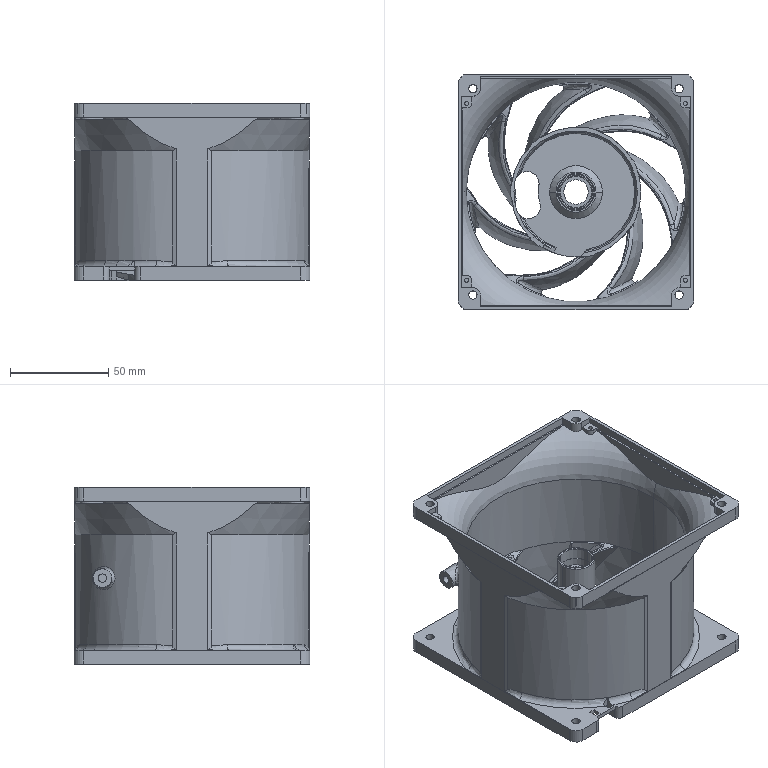NC program | NX | posted with a generic post | part box 120 x 120 x 90.2 mm
Lines 114333 to 115554 of 828686:
(等高精加工_COPY_COPY_COPY_COPY , TOOL : 2R0.2-柄4)
N228646 T09 M6
N228648 G54
N228650 G17 G0 G90 X-56.5 Y-45.575 S8000 M3
N228652 G43 Z140.7 H9
N228654 Z91.49
N228656 G94 G1 Z90.49 F1500.
N228658 X-56.759 Y-45.609
N228660 X-57. Y-45.709
N228662 X-57.207 Y-45.868
N228664 X-57.366 Y-46.075
N228666 X-57.466 Y-46.316
N228668 X-57.5 Y-46.575
N228670 Y-47.7
N228672 X-56.375
N228674 X-56.288 Z90.455
N228676 X-56.201 Z90.42
N228678 X-57.5
N228680 Y-46.401
N228682 Z90.35
N228684 Y-47.7
N228686 X-56.201
N228688 Z90.28
N228690 X-57.5
N228692 Y-46.401
N228694 Z90.21
N228696 Y-47.7
N228698 X-56.201
N228700 Z90.14
N228702 X-57.5
N228704 Y-46.401
N228706 Z90.07
N228708 Y-47.7
N228710 X-56.201
N228712 Z90.
N228714 X-57.5
N228716 Y-46.401
N228718 Z89.93
N228720 Y-47.7
N228722 X-56.201
N228724 Z89.86
N228726 X-57.5
N228728 Y-46.401
N228730 Z89.79
N228732 Y-47.7
N228734 X-56.201
N228736 Z89.72
N228738 X-57.5
N228740 Y-46.401
N228742 Z89.65
N228744 Y-47.7
N228746 X-56.201
N228748 Z89.58
N228750 X-57.5
N228752 Y-46.401
N228754 Z89.51
N228756 Y-47.7
N228758 X-56.201
N228760 Z89.44
N228762 X-57.5
N228764 Y-46.401
N228766 Z89.37
N228768 Y-47.7
N228770 X-56.201
N228772 Z89.3
N228774 X-57.5
N228776 Y-46.401
N228778 Z89.23
N228780 Y-47.7
N228782 X-56.201
N228784 Z89.16
N228786 X-57.5
N228788 Y-46.401
N228790 Z89.09
N228792 Y-47.7
N228794 X-56.201
N228796 Z89.02
N228798 X-57.5
N228800 Y-46.401
N228802 Z88.95
N228804 Y-47.7
N228806 X-56.201
N228808 Z88.88
N228810 X-57.5
N228812 Y-46.401
N228814 Z88.81
N228816 Y-47.7
N228818 X-56.201
N228820 Z88.74
N228822 X-57.5
N228824 Y-46.401
N228826 Z88.67
N228828 Y-47.7
N228830 X-56.201
N228832 Z88.6
N228834 X-57.5
N228836 Y-46.401
N228838 Z88.53
N228840 Y-47.7
N228842 X-56.201
N228844 Z88.46
N228846 X-57.5
N228848 Y-46.401
N228850 Z88.39
N228852 Y-47.7
N228854 X-56.201
N228856 Z88.32
N228858 X-57.5
N228860 Y-46.401
N228862 Z88.25
N228864 Y-47.7
N228866 X-56.201
N228868 Z88.18
N228870 X-57.5
N228872 Y-46.401
N228874 Z88.11
N228876 Y-47.7
N228878 X-56.201
N228880 Z88.04
N228882 X-57.5
N228884 Y-46.401
N228886 Z87.97
N228888 Y-47.7
N228890 X-56.201
N228892 Z87.9
N228894 X-57.5
N228896 Y-46.401
N228898 Z87.83
N228900 Y-47.7
N228902 X-56.201
N228904 Z87.76
N228906 X-57.5
N228908 Y-46.401
N228910 Z87.69
N228912 Y-47.7
N228914 X-56.201
N228916 Z87.62
N228918 X-57.5
N228920 Y-46.401
N228922 Z87.55
N228924 Y-47.7
N228926 X-56.201
N228928 Z87.48
N228930 X-57.5
N228932 Y-46.401
N228934 Z87.41
N228936 Y-47.7
N228938 X-56.201
N228940 Z87.34
N228942 X-57.5
N228944 Y-46.401
N228946 Z87.27
N228948 Y-47.7
N228950 X-56.201
N228952 Z87.2
N228954 X-57.5
N228956 Y-46.401
N228958 Z87.173
N228960 Y-47.7
N228962 X-56.201
N228964 Z87.125
N228966 X-57.5
N228968 Y-46.401
N228970 Z87.063
N228972 Y-47.7
N228974 X-56.201
N228976 Z86.994
N228978 X-57.5
N228980 Y-46.401
N228982 Z86.924
N228984 Y-47.7
N228986 X-56.201
N228988 Z86.854
N228990 X-57.5
N228992 Y-46.401
N228994 Z86.784
N228996 Y-47.7
N228998 X-56.201
N229000 Z86.714
N229002 X-57.5
N229004 Y-46.401
N229006 Z86.644
N229008 Y-47.7
N229010 X-56.201
N229012 X-55.942 Y-47.666
N229014 X-55.701 Y-47.566
N229016 X-55.494 Y-47.407
N229018 X-55.335 Y-47.2
N229020 X-55.235 Y-46.959
N229022 X-55.201 Y-46.7
N229024 Z87.644
N229026 G0 Z140.7
N229028 X-46.7 Y-55.375
N229030 Z91.49
N229032 G1 Z90.49
N229034 X-46.959 Y-55.409
N229036 X-47.2 Y-55.509
N229038 X-47.407 Y-55.668
N229040 X-47.566 Y-55.875
N229042 X-47.666 Y-56.116
N229044 X-47.7 Y-56.375
N229046 Y-57.5
N229048 X-46.575
N229050 X-46.488 Y-57.501 Z90.455
N229052 X-46.401 Y-57.5 Z90.42
N229054 X-47.7
N229056 Y-56.201
N229058 Z90.35
N229060 Y-57.5
N229062 X-46.401
N229064 Z90.28
N229066 X-47.7
N229068 Y-56.201
N229070 Z90.21
N229072 Y-57.5
N229074 X-46.401
N229076 Z90.14
N229078 X-47.7
N229080 Y-56.201
N229082 Z90.07
N229084 Y-57.5
N229086 X-46.401
N229088 Z90.
N229090 X-47.7
N229092 Y-56.201
N229094 Z89.93
N229096 Y-57.5
N229098 X-46.401
N229100 Z89.86
N229102 X-47.7
N229104 Y-56.201
N229106 Z89.79
N229108 Y-57.5
N229110 X-46.401
N229112 Z89.72
N229114 X-47.7
N229116 Y-56.201
N229118 Z89.65
N229120 Y-57.5
N229122 X-46.401
N229124 Z89.58
N229126 X-47.7
N229128 Y-56.201
N229130 Z89.51
N229132 Y-57.5
N229134 X-46.401
N229136 Z89.44
N229138 X-47.7
N229140 Y-56.201
N229142 Z89.37
N229144 Y-57.5
N229146 X-46.401
N229148 Z89.3
N229150 X-47.7
N229152 Y-56.201
N229154 Z89.23
N229156 Y-57.5
N229158 X-46.401
N229160 Z89.16
N229162 X-47.7
N229164 Y-56.201
N229166 Z89.09
N229168 Y-57.5
N229170 X-46.401
N229172 Z89.02
N229174 X-47.7
N229176 Y-56.201
N229178 Z88.95
N229180 Y-57.5
N229182 X-46.401
N229184 Z88.88
N229186 X-47.7
N229188 Y-56.201
N229190 Z88.81
N229192 Y-57.5
N229194 X-46.401
N229196 Z88.74
N229198 X-47.7
N229200 Y-56.201
N229202 Z88.67
N229204 Y-57.5
N229206 X-46.401
N229208 Z88.6
N229210 X-47.7
N229212 Y-56.201
N229214 Z88.53
N229216 Y-57.5
N229218 X-46.401
N229220 Z88.46
N229222 X-47.7
N229224 Y-56.201
N229226 Z88.39
N229228 Y-57.5
N229230 X-46.401
N229232 Z88.32
N229234 X-47.7
N229236 Y-56.201
N229238 Z88.25
N229240 Y-57.5
N229242 X-46.401
N229244 Z88.18
N229246 X-47.7
N229248 Y-56.201
N229250 Z88.11
N229252 Y-57.5
N229254 X-46.401
N229256 Z88.04
N229258 X-47.7
N229260 Y-56.201
N229262 Z87.97
N229264 Y-57.5
N229266 X-46.401
N229268 Z87.9
N229270 X-47.7
N229272 Y-56.201
N229274 Z87.83
N229276 Y-57.5
N229278 X-46.401
N229280 Z87.76
N229282 X-47.7
N229284 Y-56.201
N229286 Z87.69
N229288 Y-57.5
N229290 X-46.401
N229292 X-46.142 Y-57.466
N229294 X-45.901 Y-57.366
N229296 X-45.694 Y-57.207
N229298 X-45.535 Y-57.
N229300 X-45.435 Y-56.759
N229302 X-45.401 Y-56.5
N229304 Z88.69
N229306 G0 Z93.7
N229308 X-40.038
N229310 Z88.62
N229312 G1 Z87.62
N229314 X-40.072 Y-56.759
N229316 X-40.172 Y-57.
N229318 X-40.331 Y-57.207
N229320 X-40.538 Y-57.366
N229322 X-40.779 Y-57.466
N229324 X-41.038 Y-57.5
N229326 X-47.7
N229328 Y-52.7
N229330 X-47.734 Y-52.122
N229332 X-47.834 Y-51.552
N229334 X-47.851 Y-51.48 Z87.585
N229336 X-47.87 Y-51.409 Z87.55
N229338 X-47.776 Y-51.834
N229340 X-47.719 Y-52.265
N229342 X-47.7 Y-52.7
N229344 Y-57.5
N229346 X-40.865
N229348 X-40.78 Z87.48
N229350 X-47.7
N229352 Y-52.7
N229354 X-47.722 Y-52.232
N229356 X-47.788 Y-51.767
N229358 X-47.897 Y-51.311
N229360 X-47.918 Y-51.24 Z87.445
N229362 X-47.94 Y-51.17 Z87.41
N229364 X-47.807 Y-51.671
N229366 X-47.727 Y-52.183
N229368 X-47.7 Y-52.7
N229370 Y-57.5
N229372 X-40.63
N229374 X-40.544 Z87.34
N229376 X-47.7
N229378 Y-52.7
N229380 X-47.729 Y-52.158
N229382 X-47.817 Y-51.622
N229384 X-47.963 Y-51.1
N229386 X-47.979 Y-51.053 Z87.27
N229388 X-47.825 Y-51.59
N229390 X-47.731 Y-52.142
N229392 X-47.7 Y-52.7
N229394 Y-57.5
N229396 X-40.487
N229398 X-40.447 Z87.2
N229400 X-47.7
N229402 Y-52.7
N229404 X-47.733 Y-52.13
N229406 X-47.83 Y-51.568
N229408 X-47.991 Y-51.02
N229410 Z87.173
N229412 X-47.833 Y-51.553
N229414 X-47.736 Y-52.099
N229416 X-46.951
N229418 X-46.856 Y-52.067 Z87.149
N229420 X-46.761 Y-52.044 Z87.125
N229422 X-47.743
N229424 X-47.843 Y-51.515
N229426 X-47.998 Y-50.999
N229428 X-48.003 Y-50.987 Z87.063
N229430 X-47.848 Y-51.492
N229432 X-47.748 Y-52.01
N229434 X-46.814
N229436 X-46.823 Y-52. Z86.994
N229438 X-47.749
N229440 X-47.85 Y-51.485
N229442 X-48.004 Y-50.983
N229444 Z86.924
N229446 X-47.85 Y-51.485
N229448 X-47.749 Y-52.
N229450 X-46.647
N229452 Z86.854
N229454 X-47.749
N229456 X-47.85 Y-51.485
N229458 X-48.004 Y-50.983
N229460 Z86.784
N229462 X-47.85 Y-51.485
N229464 X-47.749 Y-52.
N229466 X-46.647
N229468 Z86.714
N229470 X-47.749
N229472 X-47.85 Y-51.485
N229474 X-48.004 Y-50.983
N229476 Z86.644
N229478 X-47.85 Y-51.485
N229480 X-47.749 Y-52.
N229482 X-46.647
N229484 Z86.574
N229486 X-47.749
N229488 X-47.85 Y-51.485
N229490 X-48.004 Y-50.983
N229492 Z86.504
N229494 X-47.85 Y-51.485
N229496 X-47.749 Y-52.
N229498 X-46.647
N229500 Z86.434
N229502 X-47.749
N229504 X-47.85 Y-51.485
N229506 X-48.004 Y-50.983
N229508 Z86.375
N229510 X-47.85 Y-51.485
N229512 X-47.749 Y-52.
N229514 X-46.647
N229516 Z86.317
N229518 X-47.749
N229520 X-47.85 Y-51.485
N229522 X-48.004 Y-50.983
N229524 Z86.258
N229526 X-47.85 Y-51.485
N229528 X-47.749 Y-52.
N229530 X-46.647
N229532 Z86.2
N229534 X-47.749
N229536 X-47.85 Y-51.485
N229538 X-48.004 Y-50.983
N229540 Z86.161
N229542 X-47.85 Y-51.485
N229544 X-47.749 Y-52.
N229546 X-46.647
N229548 Z86.108
N229550 X-47.749
N229552 X-47.85 Y-51.485
N229554 X-48.004 Y-50.983
N229556 Z86.043
N229558 X-47.85 Y-51.485
N229560 X-47.749 Y-52.
N229562 X-46.647
N229564 Z86.019
N229566 X-47.749
N229568 X-47.85 Y-51.485
N229570 X-48.004 Y-50.983
N229572 Z86.014
N229574 X-47.85 Y-51.485
N229576 X-47.749 Y-52.
N229578 X-46.647
N229580 Z86.01
N229582 X-47.749
N229584 X-47.85 Y-51.485
N229586 X-48.004 Y-50.983
N229588 Z86.005
N229590 X-47.85 Y-51.485
N229592 X-47.749 Y-52.
N229594 X-46.647
N229596 Z86.
N229598 X-47.749
N229600 X-47.85 Y-51.485
N229602 X-48.004 Y-50.983
N229604 Z85.995
N229606 X-47.85 Y-51.485
N229608 X-47.749 Y-52.
N229610 X-46.647
N229612 Z85.99
N229614 X-47.749
N229616 X-47.85 Y-51.485
N229618 X-48.004 Y-50.983
N229620 Z85.984
N229622 X-47.85 Y-51.485
N229624 X-47.749 Y-52.
N229626 X-46.647
N229628 Z85.978
N229630 X-47.749
N229632 X-47.85 Y-51.485
N229634 X-48.004 Y-50.983
N229636 Z85.972
N229638 X-47.85 Y-51.485
N229640 X-47.749 Y-52.
N229642 X-46.647
N229644 Z85.966
N229646 X-47.749
N229648 X-47.85 Y-51.485
N229650 X-48.004 Y-50.983
N229652 Z85.959
N229654 X-47.85 Y-51.485
N229656 X-47.749 Y-52.
N229658 X-46.647
N229660 Z85.952
N229662 X-47.749
N229664 X-47.85 Y-51.485
N229666 X-48.004 Y-50.983
N229668 Z85.945
N229670 X-47.85 Y-51.485
N229672 X-47.749 Y-52.
N229674 X-46.647
N229676 Z85.938
N229678 X-47.749
N229680 X-47.85 Y-51.485
N229682 X-48.004 Y-50.983
N229684 Z85.93
N229686 X-47.85 Y-51.485
N229688 X-47.749 Y-52.
N229690 X-46.647
N229692 Z85.922
N229694 X-47.749
N229696 X-47.85 Y-51.485
N229698 X-48.004 Y-50.983
N229700 Z85.914
N229702 X-47.85 Y-51.485
N229704 X-47.749 Y-52.
N229706 X-46.647
N229708 Z85.906
N229710 X-47.749
N229712 X-47.85 Y-51.485
N229714 X-48.004 Y-50.983
N229716 Z85.898
N229718 X-47.85 Y-51.485
N229720 X-47.749 Y-52.
N229722 X-46.647
N229724 Z85.889
N229726 X-47.749
N229728 X-47.85 Y-51.485
N229730 X-48.004 Y-50.983
N229732 Z85.88
N229734 X-47.85 Y-51.485
N229736 X-47.749 Y-52.
N229738 X-46.647
N229740 Z85.87
N229742 X-47.749
N229744 X-47.85 Y-51.485
N229746 X-48.004 Y-50.983
N229748 Z85.861
N229750 X-47.85 Y-51.485
N229752 X-47.749 Y-52.
N229754 X-46.647
N229756 Z85.851
N229758 X-47.749
N229760 X-47.85 Y-51.485
N229762 X-48.004 Y-50.983
N229764 Z85.841
N229766 X-47.85 Y-51.485
N229768 X-47.749 Y-52.
N229770 X-46.647
N229772 Z85.831
N229774 X-47.749
N229776 X-47.85 Y-51.485
N229778 X-48.004 Y-50.983
N229780 Z85.821
N229782 X-47.85 Y-51.485
N229784 X-47.749 Y-52.
N229786 X-46.647
N229788 Z85.81
N229790 X-47.749
N229792 X-47.85 Y-51.485
N229794 X-48.004 Y-50.983
N229796 Z85.799
N229798 X-47.85 Y-51.485
N229800 X-47.749 Y-52.
N229802 X-46.647
N229804 Z85.788
N229806 X-47.749
N229808 X-47.85 Y-51.485
N229810 X-48.004 Y-50.983
N229812 Z85.776
N229814 X-47.85 Y-51.485
N229816 X-47.749 Y-52.
N229818 X-46.647
N229820 Z85.765
N229822 X-47.749
N229824 X-47.85 Y-51.485
N229826 X-48.004 Y-50.983
N229828 Z85.753
N229830 X-47.85 Y-51.485
N229832 X-47.749 Y-52.
N229834 X-46.647
N229836 Z85.741
N229838 X-47.749
N229840 X-47.85 Y-51.485
N229842 X-48.004 Y-50.983
N229844 Z85.728
N229846 X-47.85 Y-51.485
N229848 X-47.749 Y-52.
N229850 X-46.647
N229852 Z85.716
N229854 X-47.749
N229856 X-47.85 Y-51.485
N229858 X-48.004 Y-50.983
N229860 X-48.008 Y-50.972 Z85.703
N229862 X-47.851 Y-51.479
N229864 X-47.749 Y-52.
N229866 X-46.636
N229868 X-46.587 Z85.69
N229870 X-47.749
N229872 X-47.858 Y-51.452
N229874 X-48.027 Y-50.92
N229876 X-48.048 Y-50.866 Z85.683
N229878 X-48.07 Y-50.812 Z85.676
N229880 X-47.873 Y-51.396
N229882 X-47.749 Y-52.
N229884 X-46.486
N229886 X-46.434 Z85.663
N229888 X-47.749
N229890 X-47.828 Y-51.576
N229892 X-47.943 Y-51.16
N229894 X-48.094 Y-50.755
N229896 X-48.12 Y-50.694 Z85.656
N229898 X-48.147 Y-50.633 Z85.649
N229900 X-47.971 Y-51.076
N229902 X-47.838 Y-51.533
N229904 X-47.749 Y-52.
N229906 X-46.326
N229908 X-46.271 Z85.635
N229910 X-47.749
N229912 X-47.844 Y-51.509
N229914 X-47.987 Y-51.031
N229916 X-48.177 Y-50.569
N229918 X-48.21 Y-50.5 Z85.628
N229920 X-48.245 Y-50.431 Z85.621
N229922 X-48.022 Y-50.935
N229924 X-47.856 Y-51.46
N229926 X-47.749 Y-52.
N229928 X-46.158
N229930 X-46.1 Z85.606
N229932 X-47.749
N229934 X-47.863 Y-51.433
N229936 X-48.042 Y-50.883
N229938 X-48.283 Y-50.357
N229940 X-48.325 Y-50.279 Z85.591
N229942 X-48.064 Y-50.828
N229944 X-47.871 Y-51.404
N229946 X-47.749 Y-52.
N229948 X-46.041
N229950 X-45.921 Z85.576
N229952 X-47.749
N229954 X-47.845 Y-51.504
N229956 X-47.99 Y-51.021
N229958 X-48.184 Y-50.555
N229960 X-48.423 Y-50.11
N229962 X-48.451 Y-50.064 Z85.569
N229964 X-48.481 Y-50.017 Z85.561
N229966 X-48.219 Y-50.481
N229968 X-48.009 Y-50.97
N229970 X-47.852 Y-51.478
N229972 X-47.749 Y-52.
N229974 X-45.86
N229976 X-45.798 Z85.546
N229978 X-47.749
N229980 X-47.859 Y-51.449
N229982 X-48.03 Y-50.914
N229984 X-48.26 Y-50.401
N229986 X-48.546 Y-49.917
N229988 X-48.584 Y-49.862 Z85.538
N229990 X-48.622 Y-49.807 Z85.53
N229992 X-48.315 Y-50.297
N229994 X-48.067 Y-50.82
N229996 X-47.881 Y-51.367
N229998 X-47.759 Y-51.932
N230000 X-47.722 Y-51.966
N230002 X-47.685 Y-52.
N230004 X-45.735
N230006 X-45.607 Z85.514
N230008 X-47.584
N230010 X-47.681 Y-51.911
N230012 X-47.778 Y-51.822
N230014 X-47.892 Y-51.328
N230016 X-48.056 Y-50.848
N230018 X-48.267 Y-50.387
N230020 X-48.524 Y-49.95
N230022 X-48.824 Y-49.541
N230024 X-48.873 Y-49.483 Z85.508
N230026 X-48.922 Y-49.424 Z85.503
N230028 X-48.973 Y-49.367 Z85.498
N230030 X-48.641 Y-49.78
N230032 X-48.355 Y-50.226
N230034 X-48.117 Y-50.7
N230036 X-47.932 Y-51.196
N230038 X-47.799 Y-51.709
N230040 X-47.641 Y-51.855
N230042 X-47.482 Y-52.
N230044 X-45.542
N230046 X-45.283 Y-51.966
N230048 X-45.042 Y-51.866
N230050 X-44.835 Y-51.707
N230052 X-44.676 Y-51.5
N230054 X-44.576 Y-51.259
N230056 X-44.542 Y-51.
N230058 Z86.498
N230060 G0 Z140.7
N230062 X-40.799 Y-55.529
N230064 Z88.173
N230066 G1 Z87.173
N230068 X-41.058 Y-55.564
N230070 X-41.299 Y-55.663
N230072 X-41.506 Y-55.822
N230074 X-41.665 Y-56.029
N230076 X-41.765 Y-56.271
N230078 X-41.799 Y-56.529
N230080 Y-57.5
N230082 X-40.447
N230084 X-40.421 Z87.125
N230086 X-41.744
N230088 Y-56.315
N230090 X-41.71 Y-56.368 Z87.063
N230092 Y-57.5
N230094 X-40.406
N230096 X-40.401 Z86.994
N230098 X-41.7
N230100 Y-56.377
N230102 Y-56.201 Z86.924
N230104 Y-57.5
N230106 X-40.401
N230108 Z86.854
N230110 X-41.7
N230112 Y-56.201
N230114 Z86.784
N230116 Y-57.5
N230118 X-40.401
N230120 Z86.714
N230122 X-41.7
N230124 Y-56.201
N230126 Z86.644
N230128 Y-57.5
N230130 X-40.401
N230132 X-40.142 Y-57.466
N230134 X-39.901 Y-57.366
N230136 X-39.694 Y-57.207
N230138 X-39.535 Y-57.
N230140 X-39.435 Y-56.759
N230142 X-39.401 Y-56.5
N230144 Z87.644
N230146 G0 Z140.7
N230148 X45.575
N230150 Z91.49
N230152 G1 Z90.49
N230154 X45.609 Y-56.759
N230156 X45.709 Y-57.
N230158 X45.868 Y-57.207
N230160 X46.075 Y-57.366
N230162 X46.316 Y-57.466
N230164 X46.575 Y-57.5
N230166 X47.7
N230168 Y-56.375
N230170 X47.701 Y-56.288 Z90.455
N230172 X47.7 Y-56.201 Z90.42
N230174 Y-57.5
N230176 X46.401
N230178 Z90.35
N230180 X47.7
N230182 Y-56.201
N230184 Z90.28
N230186 Y-57.5
N230188 X46.401
N230190 Z90.21
N230192 X47.7
N230194 Y-56.201
N230196 Z90.14
N230198 Y-57.5
N230200 X46.401
N230202 Z90.07
N230204 X47.7
N230206 Y-56.201
N230208 Z90.
N230210 Y-57.5
N230212 X46.401
N230214 Z89.93
N230216 X47.7
N230218 Y-56.201
N230220 Z89.86
N230222 Y-57.5
N230224 X46.401
N230226 Z89.79
N230228 X47.7
N230230 Y-56.201
N230232 Z89.72
N230234 Y-57.5
N230236 X46.401
N230238 Z89.65
N230240 X47.7
N230242 Y-56.201
N230244 Z89.58
N230246 Y-57.5
N230248 X46.401
N230250 Z89.51
N230252 X47.7
N230254 Y-56.201
N230256 Z89.44
N230258 Y-57.5
N230260 X46.401
N230262 Z89.37
N230264 X47.7
N230266 Y-56.201
N230268 Z89.3
N230270 Y-57.5
N230272 X46.401
N230274 Z89.23
N230276 X47.7
N230278 Y-56.201
N230280 Z89.16
N230282 Y-57.5
N230284 X46.401
N230286 Z89.09
N230288 X47.7
N230290 Y-56.201
N230292 Z89.02
N230294 Y-57.5
N230296 X46.401
N230298 Z88.95
N230300 X47.7
N230302 Y-56.201
N230304 Z88.88
N230306 Y-57.5
N230308 X46.401
N230310 Z88.81
N230312 X47.7
N230314 Y-56.201
N230316 Z88.74
N230318 Y-57.5
N230320 X46.401
N230322 Z88.67
N230324 X47.7
N230326 Y-56.201
N230328 Z88.6
N230330 Y-57.5
N230332 X46.401
N230334 Z88.53
N230336 X47.7
N230338 Y-56.201
N230340 Z88.46
N230342 Y-57.5
N230344 X46.401
N230346 Z88.39
N230348 X47.7
N230350 Y-56.201
N230352 Z88.32
N230354 Y-57.5
N230356 X46.401
N230358 Z88.25
N230360 X47.7
N230362 Y-56.201
N230364 Z88.18
N230366 Y-57.5
N230368 X46.401
N230370 Z88.11
N230372 X47.7
N230374 Y-56.201
N230376 Z88.04
N230378 Y-57.5
N230380 X46.401
N230382 Z87.97
N230384 X47.7
N230386 Y-56.201
N230388 Z87.9
N230390 Y-57.5
N230392 X46.401
N230394 Z87.83
N230396 X47.7
N230398 Y-56.201
N230400 Z87.76
N230402 Y-57.5
N230404 X46.401
N230406 Z87.69
N230408 X47.7
N230410 Y-56.201
N230412 X47.666 Y-55.942
N230414 X47.566 Y-55.701
N230416 X47.407 Y-55.494
N230418 X47.2 Y-55.335
N230420 X46.959 Y-55.235
N230422 X46.7 Y-55.201
N230424 Z88.69
N230426 G0 Z93.7
N230428 X47.09 Y-50.349
N230430 Z88.62
N230432 G1 Z87.62
N230434 X47.334 Y-50.442
N230436 X47.546 Y-50.594
N230438 X47.711 Y-50.797
N230440 X47.818 Y-51.035
N230442 X47.86 Y-51.292
N230444 X47.834 Y-51.552
N230446 X47.734 Y-52.122
N230448 X47.7 Y-52.7
N230450 Y-57.5
N230452 X41.038
N230454 X40.952 Y-57.499 Z87.585
N230456 X40.865 Y-57.5 Z87.55
N230458 X47.7
N230460 Y-52.7
N230462 X47.719 Y-52.265
N230464 X47.776 Y-51.834
N230466 X47.87 Y-51.409
N230468 X47.883 Y-51.36 Z87.515
N230470 X47.897 Y-51.311 Z87.48
N230472 X47.788 Y-51.767
N230474 X47.722 Y-52.232
N230476 X47.7 Y-52.7
N230478 Y-57.5
N230480 X40.78
N230482 X40.705 Y-57.499 Z87.445
N230484 X40.63 Y-57.5 Z87.41
N230486 X47.7
N230488 Y-52.7
N230490 X47.727 Y-52.183
N230492 X47.807 Y-51.671
N230494 X47.94 Y-51.17
N230496 X47.963 Y-51.1 Z87.34
N230498 X47.817 Y-51.622
N230500 X47.729 Y-52.158
N230502 X47.7 Y-52.7
N230504 Y-57.5
N230506 X40.544
N230508 X40.487 Z87.27
N230510 X47.7
N230512 Y-52.7
N230514 X47.731 Y-52.142
N230516 X47.825 Y-51.59
N230518 X47.979 Y-51.053
N230520 X47.991 Y-51.02 Z87.2
N230522 X47.83 Y-51.568
N230524 X47.733 Y-52.13
N230526 X47.7 Y-52.7
N230528 Y-57.5
N230530 X40.447
N230532 X40.189 Y-57.466
N230534 X39.947 Y-57.366
N230536 X39.74 Y-57.207
N230538 X39.581 Y-57.
N230540 X39.481 Y-56.759
N230542 X39.447 Y-56.5
N230544 Z88.2
N230546 G0 Z93.7
N230548 X45.951 Y-51.099
N230550 Z88.173
N230552 G1 Z87.173
N230554 X45.986 Y-51.358
N230556 X46.085 Y-51.599
N230558 X46.244 Y-51.806
N230560 X46.451 Y-51.965
N230562 X46.693 Y-52.065
N230564 X46.951 Y-52.099
N230566 X47.736
N230568 X47.833 Y-51.553
N230570 X47.991 Y-51.02
N230572 X47.998 Y-50.999 Z87.125
N230574 X47.843 Y-51.515
N230576 X47.743 Y-52.044
N230578 X46.761
N230580 X46.814 Y-52.01 Z87.063
N230582 X47.748
N230584 X47.848 Y-51.492
N230586 X48.003 Y-50.987
N230588 X48.004 Y-50.983 Z86.994
N230590 X47.85 Y-51.485
N230592 X47.749 Y-52.
N230594 X46.823
N230596 X46.647 Z86.924
N230598 X47.749
N230600 X47.85 Y-51.485
N230602 X48.004 Y-50.983
N230604 Z86.854
N230606 X47.85 Y-51.485
N230608 X47.749 Y-52.
N230610 X46.647
N230612 Z86.784
N230614 X47.749
N230616 X47.85 Y-51.485
N230618 X48.004 Y-50.983
N230620 Z86.714
N230622 X47.85 Y-51.485
N230624 X47.749 Y-52.
N230626 X46.647
N230628 Z86.644
N230630 X47.749
N230632 X47.85 Y-51.485
N230634 X48.004 Y-50.983
N230636 Z86.574
N230638 X47.85 Y-51.485
N230640 X47.749 Y-52.
N230642 X46.647
N230644 Z86.504
N230646 X47.749
N230648 X47.85 Y-51.485
N230650 X48.004 Y-50.983
N230652 Z86.434
N230654 X47.85 Y-51.485
N230656 X47.749 Y-52.
N230658 X46.647
N230660 Z86.375
N230662 X47.749
N230664 X47.85 Y-51.485
N230666 X48.004 Y-50.983
N230668 Z86.317
N230670 X47.85 Y-51.485
N230672 X47.749 Y-52.
N230674 X46.647
N230676 Z86.258
N230678 X47.749
N230680 X47.85 Y-51.485
N230682 X48.004 Y-50.983
N230684 Z86.2
N230686 X47.85 Y-51.485
N230688 X47.749 Y-52.
N230690 X46.647
N230692 Z86.161
N230694 X47.749
N230696 X47.85 Y-51.485
N230698 X48.004 Y-50.983
N230700 Z86.108
N230702 X47.85 Y-51.485
N230704 X47.749 Y-52.
N230706 X46.647
N230708 Z86.043
N230710 X47.749
N230712 X47.85 Y-51.485
N230714 X48.004 Y-50.983
N230716 Z86.019
N230718 X47.85 Y-51.485
N230720 X47.749 Y-52.
N230722 X46.647
N230724 Z86.014
N230726 X47.749
N230728 X47.85 Y-51.485
N230730 X48.004 Y-50.983
N230732 Z86.01
N230734 X47.85 Y-51.485
N230736 X47.749 Y-52.
N230738 X46.647
N230740 Z86.005
N230742 X47.749
N230744 X47.85 Y-51.485
N230746 X48.004 Y-50.983
N230748 Z86.
N230750 X47.85 Y-51.485
N230752 X47.749 Y-52.
N230754 X46.647
N230756 Z85.995
N230758 X47.749
N230760 X47.85 Y-51.485
N230762 X48.004 Y-50.983
N230764 Z85.99
N230766 X47.85 Y-51.485
N230768 X47.749 Y-52.
N230770 X46.647
N230772 Z85.984
N230774 X47.749
N230776 X47.85 Y-51.485
N230778 X48.004 Y-50.983
N230780 Z85.978
N230782 X47.85 Y-51.485
N230784 X47.749 Y-52.
N230786 X46.647
N230788 Z85.972
N230790 X47.749
N230792 X47.85 Y-51.485
N230794 X48.004 Y-50.983
N230796 Z85.966
N230798 X47.85 Y-51.485
N230800 X47.749 Y-52.
N230802 X46.647
N230804 Z85.959
N230806 X47.749
N230808 X47.85 Y-51.485
N230810 X48.004 Y-50.983
N230812 Z85.952
N230814 X47.85 Y-51.485
N230816 X47.749 Y-52.
N230818 X46.647
N230820 Z85.945
N230822 X47.749
N230824 X47.85 Y-51.485
N230826 X48.004 Y-50.983
N230828 Z85.938
N230830 X47.85 Y-51.485
N230832 X47.749 Y-52.
N230834 X46.647
N230836 Z85.93
N230838 X47.749
N230840 X47.85 Y-51.485
N230842 X48.004 Y-50.983
N230844 Z85.922
N230846 X47.85 Y-51.485
N230848 X47.749 Y-52.
N230850 X46.647
N230852 Z85.914
N230854 X47.749
N230856 X47.85 Y-51.485
N230858 X48.004 Y-50.983
N230860 Z85.906
N230862 X47.85 Y-51.485
N230864 X47.749 Y-52.
N230866 X46.647
N230868 Z85.898
N230870 X47.749
N230872 X47.85 Y-51.485
N230874 X48.004 Y-50.983
N230876 Z85.889
N230878 X47.85 Y-51.485
N230880 X47.749 Y-52.
N230882 X46.647
N230884 Z85.88
N230886 X47.749
N230888 X47.85 Y-51.485
N230890 X48.004 Y-50.983
N230892 Z85.87
N230894 X47.85 Y-51.485
N230896 X47.749 Y-52.
N230898 X46.647
N230900 Z85.861
N230902 X47.749
N230904 X47.85 Y-51.485
N230906 X48.004 Y-50.983
N230908 Z85.851
N230910 X47.85 Y-51.485
N230912 X47.749 Y-52.
N230914 X46.647
N230916 Z85.841
N230918 X47.749
N230920 X47.85 Y-51.485
N230922 X48.004 Y-50.983
N230924 Z85.831
N230926 X47.85 Y-51.485
N230928 X47.749 Y-52.
N230930 X46.647
N230932 Z85.821
N230934 X47.749
N230936 X47.85 Y-51.485
N230938 X48.004 Y-50.983
N230940 Z85.81
N230942 X47.85 Y-51.485
N230944 X47.749 Y-52.
N230946 X46.647
N230948 Z85.799
N230950 X47.749
N230952 X47.85 Y-51.485
N230954 X48.004 Y-50.983
N230956 Z85.788
N230958 X47.85 Y-51.485
N230960 X47.749 Y-52.
N230962 X46.647
N230964 Z85.776
N230966 X47.749
N230968 X47.85 Y-51.485
N230970 X48.004 Y-50.983
N230972 Z85.765
N230974 X47.85 Y-51.485
N230976 X47.749 Y-52.
N230978 X46.647
N230980 Z85.753
N230982 X47.749
N230984 X47.85 Y-51.485
N230986 X48.004 Y-50.983
N230988 Z85.741
N230990 X47.85 Y-51.485
N230992 X47.749 Y-52.
N230994 X46.647
N230996 Z85.728
N230998 X47.749
N231000 X47.85 Y-51.485
N231002 X48.004 Y-50.983
N231004 Z85.716
N231006 X47.85 Y-51.485
N231008 X47.749 Y-52.
N231010 X46.647
N231012 X46.636 Z85.703
N231014 X47.749
N231016 X47.851 Y-51.479
N231018 X48.008 Y-50.972
N231020 X48.027 Y-50.92 Z85.69
N231022 X47.858 Y-51.452
N231024 X47.749 Y-52.
N231026 X46.587
N231028 X46.486 Z85.676
N231030 X47.749
N231032 X47.873 Y-51.396
N231034 X48.07 Y-50.812
N231036 X48.094 Y-50.755 Z85.663
N231038 X47.943 Y-51.16
N231040 X47.828 Y-51.576
N231042 X47.749 Y-52.
N231044 X46.434
N231046 X46.326 Z85.649
N231048 X47.749
N231050 X47.838 Y-51.533
N231052 X47.971 Y-51.076
N231054 X48.147 Y-50.633
N231056 X48.177 Y-50.569 Z85.635
N231058 X47.987 Y-51.031
N231060 X47.844 Y-51.509
N231062 X47.749 Y-52.
N231064 X46.271
N231066 X46.158 Z85.621
N231068 X47.749
N231070 X47.856 Y-51.46
N231072 X48.022 Y-50.935
N231074 X48.245 Y-50.431
N231076 X48.283 Y-50.357 Z85.606
N231078 X48.042 Y-50.883
N231080 X47.863 Y-51.433
N231082 X47.749 Y-52.